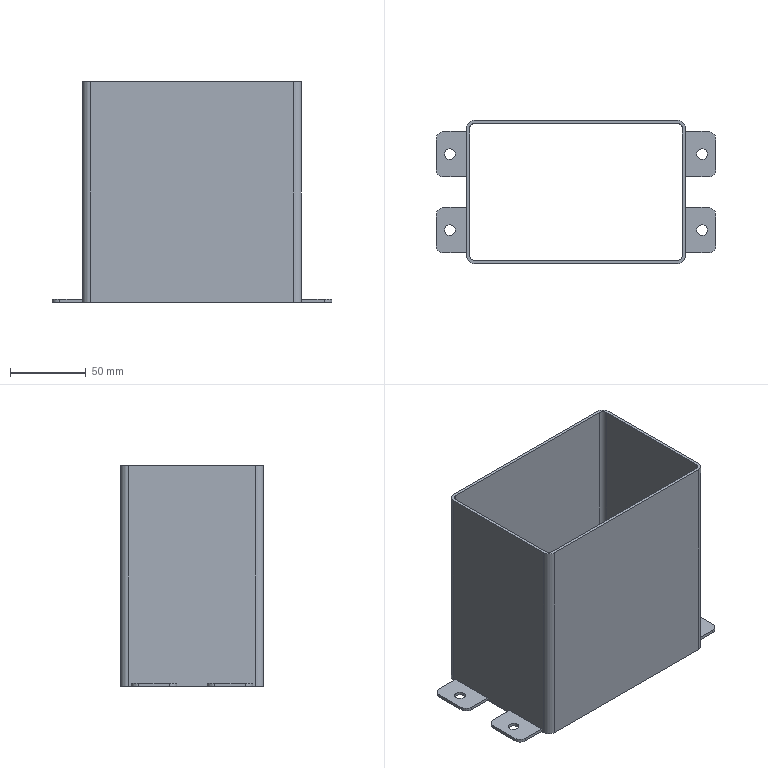Part | SolidWorks | features BaseBody 5 | 5 solids | 58 faces | box 184 x 94 x 145 mm | volume 138135 mm3 | plane 34 | cylinder 24 | commonest cylinder face diameters 10 x12 7 x8 6 x4